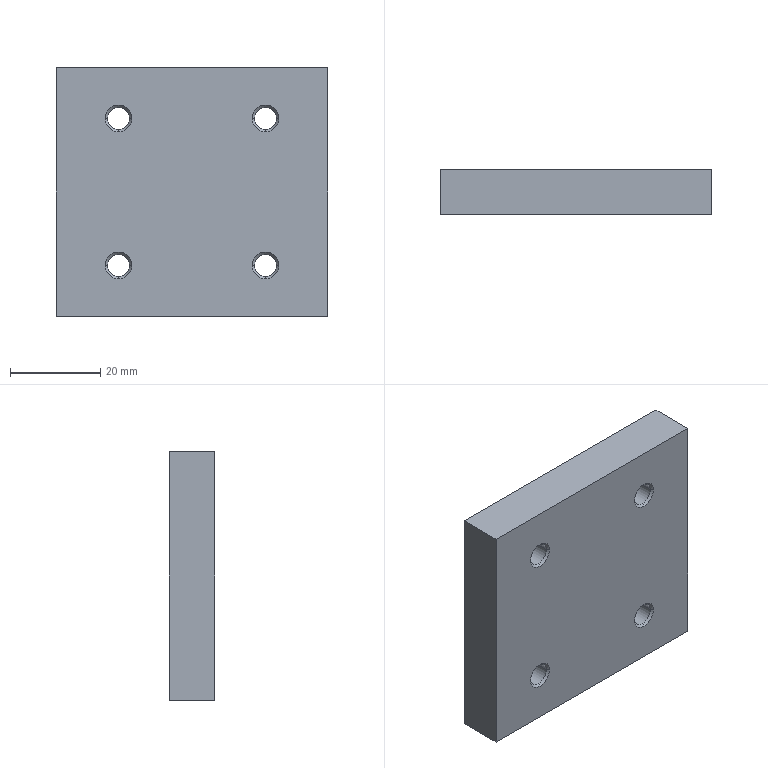Part | STEP file | 555_4 | 1 solid | 47 faces | box 60 x 10 x 54.9 mm | volume 31707 mm3 | cone 27 | cylinder 12 | plane 8 | commonest cylinder face diameters 4.917 x8 6 x4